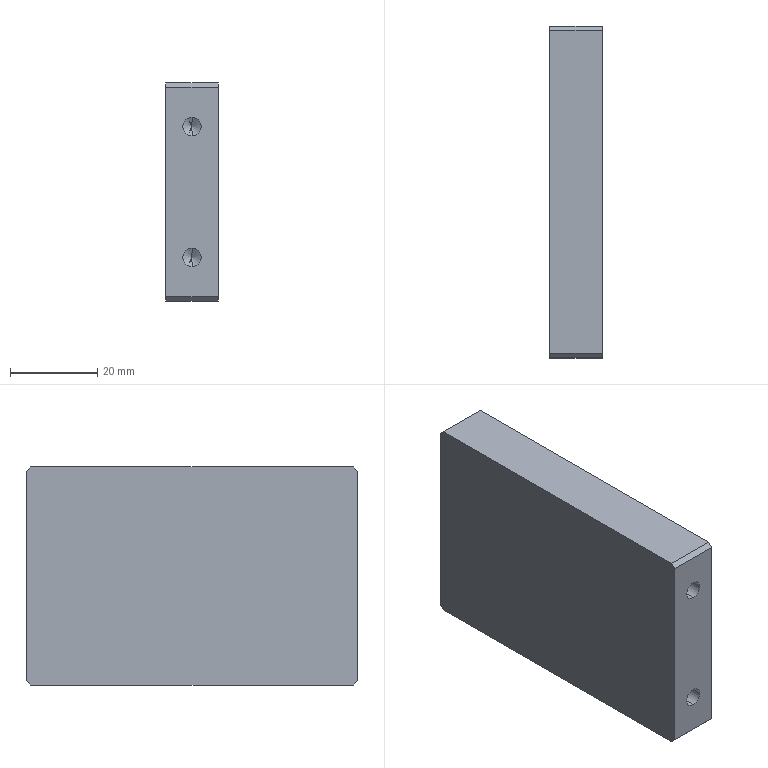Part | SolidWorks | features HoleWzd 3, Chamfer 1, ICE 1, MirrorPattern 1 | 1 solid | 26 faces | box 12 x 76 x 50 mm | volume 44588 mm3 | plane 10 | cylinder 8 | cone 8 | commonest cylinder face diameters 4.2 x8
STEP:
#1=CARTESIAN_POINT('',(-6.,20.6,-12.1));
#2=VERTEX_POINT('',#1);
#3=CARTESIAN_POINT('',(-6.,20.6,-7.9));
#4=VERTEX_POINT('',#3);
#5=CARTESIAN_POINT('',(-6.,20.6,-10.));
#6=DIRECTION('',(0.,1.,0.));
#7=DIRECTION('',(0.,0.,1.));
#8=AXIS2_PLACEMENT_3D('',#5,#6,#7);
#9=CIRCLE('',#8,2.1);
#10=EDGE_CURVE('',#2,#4,#9,.T.);
#11=ORIENTED_EDGE('',*,*,#10,.F.);
#12=CARTESIAN_POINT('',(-6.,38.,-12.1));
#13=VERTEX_POINT('',#12);
#14=CARTESIAN_POINT('',(-6.,38.,-12.1));
#15=DIRECTION('',(0.,1.,0.));
#16=VECTOR('',#15,1000.);
#17=LINE('',#14,#16);
#18=EDGE_CURVE('',#2,#13,#17,.T.);
#19=ORIENTED_EDGE('',*,*,#18,.T.);
#20=CARTESIAN_POINT('',(-6.,38.,-7.9));
#21=VERTEX_POINT('',#20);
#22=CARTESIAN_POINT('',(-6.,38.,-10.));
#23=DIRECTION('',(0.,1.,0.));
#24=DIRECTION('',(0.,0.,1.));
#25=AXIS2_PLACEMENT_3D('',#22,#23,#24);
#26=CIRCLE('',#25,2.1);
#27=EDGE_CURVE('',#13,#21,#26,.T.);
#28=ORIENTED_EDGE('',*,*,#27,.T.);
#29=CARTESIAN_POINT('',(-6.,38.,-7.9));
#30=DIRECTION('',(0.,1.,0.));
#31=VECTOR('',#30,1000.);
#32=LINE('',#29,#31);
#33=EDGE_CURVE('',#4,#21,#32,.T.);
#34=ORIENTED_EDGE('',*,*,#33,.F.);
#35=EDGE_LOOP('',(#11,#19,#28,#34));
#36=FACE_OUTER_BOUND('',#35,.T.);
#37=CARTESIAN_POINT('',(-6.,38.,-10.));
#38=DIRECTION('',(0.,1.,0.));
#39=DIRECTION('',(0.,0.,1.));
#40=AXIS2_PLACEMENT_3D('',#37,#38,#39);
#41=CYLINDRICAL_SURFACE('',#40,2.1);
#42=ADVANCED_FACE('',(#36),#41,.F.);
#43=CARTESIAN_POINT('',(-6.,19.338,-10.));
#44=VERTEX_POINT('',#43);
#45=CARTESIAN_POINT('',(-6.,20.6,-7.9));
#46=DIRECTION('',(0.,0.515,0.8572));
#47=VECTOR('',#46,1000.);
#48=LINE('',#45,#47);
#49=EDGE_CURVE('',#44,#4,#48,.T.);
#50=ORIENTED_EDGE('',*,*,#49,.F.);
#51=CARTESIAN_POINT('',(-6.,20.6,-12.1));
#52=DIRECTION('',(0.,0.515,-0.8572));
#53=VECTOR('',#52,1000.);
#54=LINE('',#51,#53);
#55=EDGE_CURVE('',#44,#2,#54,.T.);
#56=ORIENTED_EDGE('',*,*,#55,.T.);
#57=ORIENTED_EDGE('',*,*,#10,.T.);
#58=EDGE_LOOP('',(#50,#56,#57));
#59=FACE_OUTER_BOUND('',#58,.T.);
#60=CARTESIAN_POINT('',(-6.,20.6,-10.));
#61=DIRECTION('',(0.,1.,0.));
#62=DIRECTION('',(0.,0.,1.));
#63=AXIS2_PLACEMENT_3D('',#60,#61,#62);
#64=CONICAL_SURFACE('',#63,2.1,1.03);
#65=ADVANCED_FACE('',(#59),#64,.F.);
#66=CARTESIAN_POINT('',(-6.,20.6,-42.1));
#67=VERTEX_POINT('',#66);
#68=CARTESIAN_POINT('',(-6.,20.6,-37.9));
#69=VERTEX_POINT('',#68);
#70=CARTESIAN_POINT('',(-6.,20.6,-40.));
#71=DIRECTION('',(0.,1.,0.));
#72=DIRECTION('',(0.,0.,1.));
#73=AXIS2_PLACEMENT_3D('',#70,#71,#72);
#74=CIRCLE('',#73,2.1);
#75=EDGE_CURVE('',#67,#69,#74,.T.);
#76=ORIENTED_EDGE('',*,*,#75,.F.);
#77=CARTESIAN_POINT('',(-6.,38.,-42.1));
#78=VERTEX_POINT('',#77);
#79=CARTESIAN_POINT('',(-6.,38.,-42.1));
#80=DIRECTION('',(0.,1.,0.));
#81=VECTOR('',#80,1000.);
#82=LINE('',#79,#81);
#83=EDGE_CURVE('',#67,#78,#82,.T.);
#84=ORIENTED_EDGE('',*,*,#83,.T.);
#85=CARTESIAN_POINT('',(-6.,38.,-37.9));
#86=VERTEX_POINT('',#85);
#87=CARTESIAN_POINT('',(-6.,38.,-40.));
#88=DIRECTION('',(0.,1.,0.));
#89=DIRECTION('',(0.,0.,1.));
#90=AXIS2_PLACEMENT_3D('',#87,#88,#89);
#91=CIRCLE('',#90,2.1);
#92=EDGE_CURVE('',#78,#86,#91,.T.);
#93=ORIENTED_EDGE('',*,*,#92,.T.);
#94=CARTESIAN_POINT('',(-6.,38.,-37.9));
#95=DIRECTION('',(0.,1.,0.));
#96=VECTOR('',#95,1000.);
#97=LINE('',#94,#96);
#98=EDGE_CURVE('',#69,#86,#97,.T.);
#99=ORIENTED_EDGE('',*,*,#98,.F.);
#100=EDGE_LOOP('',(#76,#84,#93,#99));
#101=FACE_OUTER_BOUND('',#100,.T.);
#102=CARTESIAN_POINT('',(-6.,38.,-40.));
#103=DIRECTION('',(0.,1.,0.));
#104=DIRECTION('',(0.,0.,1.));
#105=AXIS2_PLACEMENT_3D('',#102,#103,#104);
#106=CYLINDRICAL_SURFACE('',#105,2.1);
#107=ADVANCED_FACE('',(#101),#106,.F.);
#108=CARTESIAN_POINT('',(-6.,19.338,-40.));
#109=VERTEX_POINT('',#108);
#110=CARTESIAN_POINT('',(-6.,20.6,-37.9));
#111=DIRECTION('',(0.,0.515,0.8572));
#112=VECTOR('',#111,1000.);
#113=LINE('',#110,#112);
#114=EDGE_CURVE('',#109,#69,#113,.T.);
#115=ORIENTED_EDGE('',*,*,#114,.F.);
#116=CARTESIAN_POINT('',(-6.,20.6,-42.1));
#117=DIRECTION('',(0.,0.515,-0.8572));
#118=VECTOR('',#117,1000.);
#119=LINE('',#116,#118);
#120=EDGE_CURVE('',#109,#67,#119,.T.);
#121=ORIENTED_EDGE('',*,*,#120,.T.);
#122=ORIENTED_EDGE('',*,*,#75,.T.);
#123=EDGE_LOOP('',(#115,#121,#122));
#124=FACE_OUTER_BOUND('',#123,.T.);
#125=CARTESIAN_POINT('',(-6.,20.6,-40.));
#126=DIRECTION('',(0.,1.,0.));
#127=DIRECTION('',(0.,0.,1.));
#128=AXIS2_PLACEMENT_3D('',#125,#126,#127);
#129=CONICAL_SURFACE('',#128,2.1,1.03);
#130=ADVANCED_FACE('',(#124),#129,.F.);
#131=CARTESIAN_POINT('',(-6.,-20.6,-7.9));
#132=VERTEX_POINT('',#131);
#133=CARTESIAN_POINT('',(-6.,-20.6,-12.1));
#134=VERTEX_POINT('',#133);
#135=CARTESIAN_POINT('',(-6.,-20.6,-10.));
#136=DIRECTION('',(0.,-1.,0.));
#137=DIRECTION('',(0.,0.,-1.));
#138=AXIS2_PLACEMENT_3D('',#135,#136,#137);
#139=CIRCLE('',#138,2.1);
#140=EDGE_CURVE('',#132,#134,#139,.T.);
#141=ORIENTED_EDGE('',*,*,#140,.F.);
#142=CARTESIAN_POINT('',(-6.,-38.,-7.9));
#143=VERTEX_POINT('',#142);
#144=CARTESIAN_POINT('',(-6.,-38.,-7.9));
#145=DIRECTION('',(0.,-1.,0.));
#146=VECTOR('',#145,1000.);
#147=LINE('',#144,#146);
#148=EDGE_CURVE('',#132,#143,#147,.T.);
#149=ORIENTED_EDGE('',*,*,#148,.T.);
#150=CARTESIAN_POINT('',(-6.,-38.,-12.1));
#151=VERTEX_POINT('',#150);
#152=CARTESIAN_POINT('',(-6.,-38.,-10.));
#153=DIRECTION('',(0.,-1.,0.));
#154=DIRECTION('',(0.,0.,-1.));
#155=AXIS2_PLACEMENT_3D('',#152,#153,#154);
#156=CIRCLE('',#155,2.1);
#157=EDGE_CURVE('',#143,#151,#156,.T.);
#158=ORIENTED_EDGE('',*,*,#157,.T.);
#159=CARTESIAN_POINT('',(-6.,-38.,-12.1));
#160=DIRECTION('',(0.,-1.,0.));
#161=VECTOR('',#160,1000.);
#162=LINE('',#159,#161);
#163=EDGE_CURVE('',#134,#151,#162,.T.);
#164=ORIENTED_EDGE('',*,*,#163,.F.);
#165=EDGE_LOOP('',(#141,#149,#158,#164));
#166=FACE_OUTER_BOUND('',#165,.T.);
#167=CARTESIAN_POINT('',(-6.,-38.,-10.));
#168=DIRECTION('',(0.,-1.,0.));
#169=DIRECTION('',(0.,0.,-1.));
#170=AXIS2_PLACEMENT_3D('',#167,#168,#169);
#171=CYLINDRICAL_SURFACE('',#170,2.1);
#172=ADVANCED_FACE('',(#166),#171,.F.);
#173=CARTESIAN_POINT('',(-6.,-19.338,-10.));
#174=VERTEX_POINT('',#173);
#175=CARTESIAN_POINT('',(-6.,-20.6,-12.1));
#176=DIRECTION('',(0.,-0.515,-0.8572));
#177=VECTOR('',#176,1000.);
#178=LINE('',#175,#177);
#179=EDGE_CURVE('',#174,#134,#178,.T.);
#180=ORIENTED_EDGE('',*,*,#179,.F.);
#181=CARTESIAN_POINT('',(-6.,-20.6,-7.9));
#182=DIRECTION('',(0.,-0.515,0.8572));
#183=VECTOR('',#182,1000.);
#184=LINE('',#181,#183);
#185=EDGE_CURVE('',#174,#132,#184,.T.);
#186=ORIENTED_EDGE('',*,*,#185,.T.);
#187=ORIENTED_EDGE('',*,*,#140,.T.);
#188=EDGE_LOOP('',(#180,#186,#187));
#189=FACE_OUTER_BOUND('',#188,.T.);
#190=CARTESIAN_POINT('',(-6.,-20.6,-10.));
#191=DIRECTION('',(0.,-1.,0.));
#192=DIRECTION('',(0.,0.,-1.));
#193=AXIS2_PLACEMENT_3D('',#190,#191,#192);
#194=CONICAL_SURFACE('',#193,2.1,1.03);
#195=ADVANCED_FACE('',(#189),#194,.F.);
#196=CARTESIAN_POINT('',(-6.,-20.6,-37.9));
#197=VERTEX_POINT('',#196);
#198=CARTESIAN_POINT('',(-6.,-20.6,-42.1));
#199=VERTEX_POINT('',#198);
#200=CARTESIAN_POINT('',(-6.,-20.6,-40.));
#201=DIRECTION('',(0.,-1.,0.));
#202=DIRECTION('',(0.,0.,-1.));
#203=AXIS2_PLACEMENT_3D('',#200,#201,#202);
#204=CIRCLE('',#203,2.1);
#205=EDGE_CURVE('',#197,#199,#204,.T.);
#206=ORIENTED_EDGE('',*,*,#205,.F.);
#207=CARTESIAN_POINT('',(-6.,-38.,-37.9));
#208=VERTEX_POINT('',#207);
#209=CARTESIAN_POINT('',(-6.,-38.,-37.9));
#210=DIRECTION('',(0.,-1.,0.));
#211=VECTOR('',#210,1000.);
#212=LINE('',#209,#211);
#213=EDGE_CURVE('',#197,#208,#212,.T.);
#214=ORIENTED_EDGE('',*,*,#213,.T.);
#215=CARTESIAN_POINT('',(-6.,-38.,-42.1));
#216=VERTEX_POINT('',#215);
#217=CARTESIAN_POINT('',(-6.,-38.,-40.));
#218=DIRECTION('',(0.,-1.,0.));
#219=DIRECTION('',(0.,0.,-1.));
#220=AXIS2_PLACEMENT_3D('',#217,#218,#219);
#221=CIRCLE('',#220,2.1);
#222=EDGE_CURVE('',#208,#216,#221,.T.);
#223=ORIENTED_EDGE('',*,*,#222,.T.);
#224=CARTESIAN_POINT('',(-6.,-38.,-42.1));
#225=DIRECTION('',(0.,-1.,0.));
#226=VECTOR('',#225,1000.);
#227=LINE('',#224,#226);
#228=EDGE_CURVE('',#199,#216,#227,.T.);
#229=ORIENTED_EDGE('',*,*,#228,.F.);
#230=EDGE_LOOP('',(#206,#214,#223,#229));
#231=FACE_OUTER_BOUND('',#230,.T.);
#232=CARTESIAN_POINT('',(-6.,-38.,-40.));
#233=DIRECTION('',(0.,-1.,0.));
#234=DIRECTION('',(0.,0.,-1.));
#235=AXIS2_PLACEMENT_3D('',#232,#233,#234);
#236=CYLINDRICAL_SURFACE('',#235,2.1);
#237=ADVANCED_FACE('',(#231),#236,.F.);
#238=CARTESIAN_POINT('',(-6.,-19.338,-40.));
#239=VERTEX_POINT('',#238);
#240=CARTESIAN_POINT('',(-6.,-20.6,-42.1));
#241=DIRECTION('',(0.,-0.515,-0.8572));
#242=VECTOR('',#241,1000.);
#243=LINE('',#240,#242);
#244=EDGE_CURVE('',#239,#199,#243,.T.);
#245=ORIENTED_EDGE('',*,*,#244,.F.);
#246=CARTESIAN_POINT('',(-6.,-20.6,-37.9));
#247=DIRECTION('',(0.,-0.515,0.8572));
#248=VECTOR('',#247,1000.);
#249=LINE('',#246,#248);
#250=EDGE_CURVE('',#239,#197,#249,.T.);
#251=ORIENTED_EDGE('',*,*,#250,.T.);
#252=ORIENTED_EDGE('',*,*,#205,.T.);
#253=EDGE_LOOP('',(#245,#251,#252));
#254=FACE_OUTER_BOUND('',#253,.T.);
#255=CARTESIAN_POINT('',(-6.,-20.6,-40.));
#256=DIRECTION('',(0.,-1.,0.));
#257=DIRECTION('',(0.,0.,-1.));
#258=AXIS2_PLACEMENT_3D('',#255,#256,#257);
#259=CONICAL_SURFACE('',#258,2.1,1.03);
#260=ADVANCED_FACE('',(#254),#259,.F.);
#261=CARTESIAN_POINT('',(0.,37.,0.));
#262=VERTEX_POINT('',#261);
#263=CARTESIAN_POINT('',(0.,-37.,0.));
#264=VERTEX_POINT('',#263);
#265=CARTESIAN_POINT('',(0.,38.,0.));
#266=DIRECTION('',(0.,-1.,0.));
#267=VECTOR('',#266,1000.);
#268=LINE('',#265,#267);
#269=EDGE_CURVE('',#262,#264,#268,.T.);
#270=ORIENTED_EDGE('',*,*,#269,.F.);
#271=CARTESIAN_POINT('',(-12.,37.,0.));
#272=VERTEX_POINT('',#271);
#273=CARTESIAN_POINT('',(-12.,37.,0.));
#274=DIRECTION('',(-1.,0.,0.));
#275=VECTOR('',#274,1000.);
#276=LINE('',#273,#275);
#277=EDGE_CURVE('',#262,#272,#276,.T.);
#278=ORIENTED_EDGE('',*,*,#277,.T.);
#279=CARTESIAN_POINT('',(-12.,-37.,0.));
#280=VERTEX_POINT('',#279);
#281=CARTESIAN_POINT('',(-12.,38.,0.));
#282=DIRECTION('',(0.,-1.,0.));
#283=VECTOR('',#282,1000.);
#284=LINE('',#281,#283);
#285=EDGE_CURVE('',#272,#280,#284,.T.);
#286=ORIENTED_EDGE('',*,*,#285,.T.);
#287=CARTESIAN_POINT('',(-12.,-37.,0.));
#288=DIRECTION('',(1.,0.,0.));
#289=VECTOR('',#288,1000.);
#290=LINE('',#287,#289);
#291=EDGE_CURVE('',#280,#264,#290,.T.);
#292=ORIENTED_EDGE('',*,*,#291,.T.);
#293=EDGE_LOOP('',(#270,#278,#286,#292));
#294=FACE_OUTER_BOUND('',#293,.T.);
#295=CARTESIAN_POINT('',(-12.,38.,0.));
#296=DIRECTION('',(0.,0.,1.));
#297=DIRECTION('',(1.,0.,0.));
#298=AXIS2_PLACEMENT_3D('',#295,#296,#297);
#299=PLANE('',#298);
#300=ADVANCED_FACE('',(#294),#299,.T.);
#301=CARTESIAN_POINT('',(-6.,38.,-10.));
#302=DIRECTION('',(0.,1.,0.));
#303=DIRECTION('',(0.,0.,1.));
#304=AXIS2_PLACEMENT_3D('',#301,#302,#303);
#305=CIRCLE('',#304,2.1);
#306=EDGE_CURVE('',#21,#13,#305,.T.);
#307=ORIENTED_EDGE('',*,*,#306,.F.);
#308=ORIENTED_EDGE('',*,*,#27,.F.);
#309=EDGE_LOOP('',(#307,#308));
#310=FACE_BOUND('',#309,.T.);
#311=CARTESIAN_POINT('',(-6.,38.,-40.));
#312=DIRECTION('',(0.,1.,0.));
#313=DIRECTION('',(0.,0.,1.));
#314=AXIS2_PLACEMENT_3D('',#311,#312,#313);
#315=CIRCLE('',#314,2.1);
#316=EDGE_CURVE('',#86,#78,#315,.T.);
#317=ORIENTED_EDGE('',*,*,#316,.F.);
#318=ORIENTED_EDGE('',*,*,#92,.F.);
#319=EDGE_LOOP('',(#317,#318));
#320=FACE_BOUND('',#319,.T.);
#321=CARTESIAN_POINT('',(-12.,38.,-49.));
#322=VERTEX_POINT('',#321);
#323=CARTESIAN_POINT('',(-12.,38.,-1.));
#324=VERTEX_POINT('',#323);
#325=CARTESIAN_POINT('',(-12.,38.,0.));
#326=DIRECTION('',(0.,0.,1.));
#327=VECTOR('',#326,1000.);
#328=LINE('',#325,#327);
#329=EDGE_CURVE('',#322,#324,#328,.T.);
#330=ORIENTED_EDGE('',*,*,#329,.T.);
#331=CARTESIAN_POINT('',(0.,38.,-1.));
#332=VERTEX_POINT('',#331);
#333=CARTESIAN_POINT('',(-12.,38.,-1.));
#334=DIRECTION('',(1.,0.,0.));
#335=VECTOR('',#334,1000.);
#336=LINE('',#333,#335);
#337=EDGE_CURVE('',#324,#332,#336,.T.);
#338=ORIENTED_EDGE('',*,*,#337,.T.);
#339=CARTESIAN_POINT('',(0.,38.,-49.));
#340=VERTEX_POINT('',#339);
#341=CARTESIAN_POINT('',(0.,38.,0.));
#342=DIRECTION('',(0.,0.,1.));
#343=VECTOR('',#342,1000.);
#344=LINE('',#341,#343);
#345=EDGE_CURVE('',#340,#332,#344,.T.);
#346=ORIENTED_EDGE('',*,*,#345,.F.);
#347=CARTESIAN_POINT('',(-12.,38.,-49.));
#348=DIRECTION('',(-1.,0.,0.));
#349=VECTOR('',#348,1000.);
#350=LINE('',#347,#349);
#351=EDGE_CURVE('',#340,#322,#350,.T.);
#352=ORIENTED_EDGE('',*,*,#351,.T.);
#353=EDGE_LOOP('',(#330,#338,#346,#352));
#354=FACE_OUTER_BOUND('',#353,.T.);
#355=CARTESIAN_POINT('',(-12.,38.,0.));
#356=DIRECTION('',(0.,1.,0.));
#357=DIRECTION('',(0.,0.,1.));
#358=AXIS2_PLACEMENT_3D('',#355,#356,#357);
#359=PLANE('',#358);
#360=ADVANCED_FACE('',(#310,#320,#354),#359,.T.);
#361=CARTESIAN_POINT('',(-12.,-37.,-50.));
#362=VERTEX_POINT('',#361);
#363=CARTESIAN_POINT('',(-12.,37.,-50.));
#364=VERTEX_POINT('',#363);
#365=CARTESIAN_POINT('',(-12.,38.,-50.));
#366=DIRECTION('',(0.,1.,0.));
#367=VECTOR('',#366,1000.);
#368=LINE('',#365,#367);
#369=EDGE_CURVE('',#362,#364,#368,.T.);
#370=ORIENTED_EDGE('',*,*,#369,.T.);
#371=CARTESIAN_POINT('',(0.,37.,-50.));
#372=VERTEX_POINT('',#371);
#373=CARTESIAN_POINT('',(-12.,37.,-50.));
#374=DIRECTION('',(1.,0.,0.));
#375=VECTOR('',#374,1000.);
#376=LINE('',#373,#375);
#377=EDGE_CURVE('',#364,#372,#376,.T.);
#378=ORIENTED_EDGE('',*,*,#377,.T.);
#379=CARTESIAN_POINT('',(0.,-37.,-50.));
#380=VERTEX_POINT('',#379);
#381=CARTESIAN_POINT('',(0.,38.,-50.));
#382=DIRECTION('',(0.,1.,0.));
#383=VECTOR('',#382,1000.);
#384=LINE('',#381,#383);
#385=EDGE_CURVE('',#380,#372,#384,.T.);
#386=ORIENTED_EDGE('',*,*,#385,.F.);
#387=CARTESIAN_POINT('',(-12.,-37.,-50.));
#388=DIRECTION('',(-1.,0.,0.));
#389=VECTOR('',#388,1000.);
#390=LINE('',#387,#389);
#391=EDGE_CURVE('',#380,#362,#390,.T.);
#392=ORIENTED_EDGE('',*,*,#391,.T.);
#393=EDGE_LOOP('',(#370,#378,#386,#392));
#394=FACE_OUTER_BOUND('',#393,.T.);
#395=CARTESIAN_POINT('',(-12.,38.,-50.));
#396=DIRECTION('',(0.,0.,-1.));
#397=DIRECTION('',(-1.,0.,0.));
#398=AXIS2_PLACEMENT_3D('',#395,#396,#397);
#399=PLANE('',#398);
#400=ADVANCED_FACE('',(#394),#399,.T.);
#401=CARTESIAN_POINT('',(-6.,-38.,-10.));
#402=DIRECTION('',(0.,-1.,0.));
#403=DIRECTION('',(0.,0.,-1.));
#404=AXIS2_PLACEMENT_3D('',#401,#402,#403);
#405=CIRCLE('',#404,2.1);
#406=EDGE_CURVE('',#151,#143,#405,.T.);
#407=ORIENTED_EDGE('',*,*,#406,.F.);
#408=ORIENTED_EDGE('',*,*,#157,.F.);
#409=EDGE_LOOP('',(#407,#408));
#410=FACE_BOUND('',#409,.T.);
#411=CARTESIAN_POINT('',(-6.,-38.,-40.));
#412=DIRECTION('',(0.,-1.,0.));
#413=DIRECTION('',(0.,0.,-1.));
#414=AXIS2_PLACEMENT_3D('',#411,#412,#413);
#415=CIRCLE('',#414,2.1);
#416=EDGE_CURVE('',#216,#208,#415,.T.);
#417=ORIENTED_EDGE('',*,*,#416,.F.);
#418=ORIENTED_EDGE('',*,*,#222,.F.);
#419=EDGE_LOOP('',(#417,#418));
#420=FACE_BOUND('',#419,.T.);
#421=CARTESIAN_POINT('',(-12.,-38.,-1.));
#422=VERTEX_POINT('',#421);
#423=CARTESIAN_POINT('',(-12.,-38.,-49.));
#424=VERTEX_POINT('',#423);
#425=CARTESIAN_POINT('',(-12.,-38.,0.));
#426=DIRECTION('',(0.,0.,-1.));
#427=VECTOR('',#426,1000.);
#428=LINE('',#425,#427);
#429=EDGE_CURVE('',#422,#424,#428,.T.);
#430=ORIENTED_EDGE('',*,*,#429,.T.);
#431=CARTESIAN_POINT('',(0.,-38.,-49.));
#432=VERTEX_POINT('',#431);
#433=CARTESIAN_POINT('',(-12.,-38.,-49.));
#434=DIRECTION('',(1.,0.,0.));
#435=VECTOR('',#434,1000.);
#436=LINE('',#433,#435);
#437=EDGE_CURVE('',#424,#432,#436,.T.);
#438=ORIENTED_EDGE('',*,*,#437,.T.);
#439=CARTESIAN_POINT('',(0.,-38.,-1.));
#440=VERTEX_POINT('',#439);
#441=CARTESIAN_POINT('',(0.,-38.,0.));
#442=DIRECTION('',(0.,0.,-1.));
#443=VECTOR('',#442,1000.);
#444=LINE('',#441,#443);
#445=EDGE_CURVE('',#440,#432,#444,.T.);
#446=ORIENTED_EDGE('',*,*,#445,.F.);
#447=CARTESIAN_POINT('',(-12.,-38.,-1.));
#448=DIRECTION('',(-1.,0.,0.));
#449=VECTOR('',#448,1000.);
#450=LINE('',#447,#449);
#451=EDGE_CURVE('',#440,#422,#450,.T.);
#452=ORIENTED_EDGE('',*,*,#451,.T.);
#453=EDGE_LOOP('',(#430,#438,#446,#452));
#454=FACE_OUTER_BOUND('',#453,.T.);
#455=CARTESIAN_POINT('',(-12.,-38.,0.));
#456=DIRECTION('',(0.,-1.,0.));
#457=DIRECTION('',(0.,0.,-1.));
#458=AXIS2_PLACEMENT_3D('',#455,#456,#457);
#459=PLANE('',#458);
#460=ADVANCED_FACE('',(#410,#420,#454),#459,.T.);
#461=ORIENTED_EDGE('',*,*,#285,.F.);
#462=CARTESIAN_POINT('',(-12.,38.,-1.));
#463=DIRECTION('',(0.,0.7071,-0.7071));
#464=VECTOR('',#463,1000.);
#465=LINE('',#462,#464);
#466=EDGE_CURVE('',#272,#324,#465,.T.);
#467=ORIENTED_EDGE('',*,*,#466,.T.);
#468=ORIENTED_EDGE('',*,*,#329,.F.);
#469=CARTESIAN_POINT('',(-12.,37.,-50.));
#470=DIRECTION('',(0.,-0.7071,-0.7071));
#471=VECTOR('',#470,1000.);
#472=LINE('',#469,#471);
#473=EDGE_CURVE('',#322,#364,#472,.T.);
#474=ORIENTED_EDGE('',*,*,#473,.T.);
#475=ORIENTED_EDGE('',*,*,#369,.F.);
#476=CARTESIAN_POINT('',(-12.,-38.,-49.));
#477=DIRECTION('',(0.,-0.7071,0.7071));
#478=VECTOR('',#477,1000.);
#479=LINE('',#476,#478);
#480=EDGE_CURVE('',#362,#424,#479,.T.);
#481=ORIENTED_EDGE('',*,*,#480,.T.);
#482=ORIENTED_EDGE('',*,*,#429,.F.);
#483=CARTESIAN_POINT('',(-12.,-37.,0.));
#484=DIRECTION('',(0.,0.7071,0.7071));
#485=VECTOR('',#484,1000.);
#486=LINE('',#483,#485);
#487=EDGE_CURVE('',#422,#280,#486,.T.);
#488=ORIENTED_EDGE('',*,*,#487,.T.);
#489=EDGE_LOOP('',(#461,#467,#468,#474,#475,#481,#482,#488));
#490=FACE_OUTER_BOUND('',#489,.T.);
#491=CARTESIAN_POINT('',(-12.,0.,0.));
#492=DIRECTION('',(1.,0.,0.));
#493=DIRECTION('',(0.,0.,-1.));
#494=AXIS2_PLACEMENT_3D('',#491,#492,#493);
#495=PLANE('',#494);
#496=ADVANCED_FACE('',(#490),#495,.F.);
#497=ORIENTED_EDGE('',*,*,#345,.T.);
#498=CARTESIAN_POINT('',(0.,18.5,18.5));
#499=DIRECTION('',(0.,-0.7071,0.7071));
#500=VECTOR('',#499,1000.);
#501=LINE('',#498,#500);
#502=EDGE_CURVE('',#332,#262,#501,.T.);
#503=ORIENTED_EDGE('',*,*,#502,.T.);
#504=ORIENTED_EDGE('',*,*,#269,.T.);
#505=CARTESIAN_POINT('',(0.,-18.5,18.5));
#506=DIRECTION('',(0.,-0.7071,-0.7071));
#507=VECTOR('',#506,1000.);
#508=LINE('',#505,#507);
#509=EDGE_CURVE('',#264,#440,#508,.T.);
#510=ORIENTED_EDGE('',*,*,#509,.T.);
#511=ORIENTED_EDGE('',*,*,#445,.T.);
#512=CARTESIAN_POINT('',(0.,-43.5,-43.5));
#513=DIRECTION('',(0.,0.7071,-0.7071));
#514=VECTOR('',#513,1000.);
#515=LINE('',#512,#514);
#516=EDGE_CURVE('',#432,#380,#515,.T.);
#517=ORIENTED_EDGE('',*,*,#516,.T.);
#518=ORIENTED_EDGE('',*,*,#385,.T.);
#519=CARTESIAN_POINT('',(0.,43.5,-43.5));
#520=DIRECTION('',(0.,0.7071,0.7071));
#521=VECTOR('',#520,1000.);
#522=LINE('',#519,#521);
#523=EDGE_CURVE('',#372,#340,#522,.T.);
#524=ORIENTED_EDGE('',*,*,#523,.T.);
#525=EDGE_LOOP('',(#497,#503,#504,#510,#511,#517,#518,#524));
#526=FACE_OUTER_BOUND('',#525,.T.);
#527=CARTESIAN_POINT('',(0.,0.,0.));
#528=DIRECTION('',(1.,0.,0.));
#529=DIRECTION('',(0.,0.,-1.));
#530=AXIS2_PLACEMENT_3D('',#527,#528,#529);
#531=PLANE('',#530);
#532=ADVANCED_FACE('',(#526),#531,.T.);
#533=ORIENTED_EDGE('',*,*,#250,.F.);
#534=ORIENTED_EDGE('',*,*,#244,.T.);
#535=CARTESIAN_POINT('',(-6.,-20.6,-40.));
#536=DIRECTION('',(0.,-1.,0.));
#537=DIRECTION('',(0.,0.,-1.));
#538=AXIS2_PLACEMENT_3D('',#535,#536,#537);
#539=CIRCLE('',#538,2.1);
#540=EDGE_CURVE('',#199,#197,#539,.T.);
#541=ORIENTED_EDGE('',*,*,#540,.T.);
#542=EDGE_LOOP('',(#533,#534,#541));
#543=FACE_OUTER_BOUND('',#542,.T.);
#544=CARTESIAN_POINT('',(-6.,-20.6,-40.));
#545=DIRECTION('',(0.,-1.,0.));
#546=DIRECTION('',(0.,0.,-1.));
#547=AXIS2_PLACEMENT_3D('',#544,#545,#546);
#548=CONICAL_SURFACE('',#547,2.1,1.03);
#549=ADVANCED_FACE('',(#543),#548,.F.);
#550=ORIENTED_EDGE('',*,*,#213,.F.);
#551=ORIENTED_EDGE('',*,*,#540,.F.);
#552=ORIENTED_EDGE('',*,*,#228,.T.);
#553=ORIENTED_EDGE('',*,*,#416,.T.);
#554=EDGE_LOOP('',(#550,#551,#552,#553));
#555=FACE_OUTER_BOUND('',#554,.T.);
#556=CARTESIAN_POINT('',(-6.,-38.,-40.));
#557=DIRECTION('',(0.,-1.,0.));
#558=DIRECTION('',(0.,0.,-1.));
#559=AXIS2_PLACEMENT_3D('',#556,#557,#558);
#560=CYLINDRICAL_SURFACE('',#559,2.1);
#561=ADVANCED_FACE('',(#555),#560,.F.);
#562=ORIENTED_EDGE('',*,*,#185,.F.);
#563=ORIENTED_EDGE('',*,*,#179,.T.);
#564=CARTESIAN_POINT('',(-6.,-20.6,-10.));
#565=DIRECTION('',(0.,-1.,0.));
#566=DIRECTION('',(0.,0.,-1.));
#567=AXIS2_PLACEMENT_3D('',#564,#565,#566);
#568=CIRCLE('',#567,2.1);
#569=EDGE_CURVE('',#134,#132,#568,.T.);
#570=ORIENTED_EDGE('',*,*,#569,.T.);
#571=EDGE_LOOP('',(#562,#563,#570));
#572=FACE_OUTER_BOUND('',#571,.T.);
#573=CARTESIAN_POINT('',(-6.,-20.6,-10.));
#574=DIRECTION('',(0.,-1.,0.));
#575=DIRECTION('',(0.,0.,-1.));
#576=AXIS2_PLACEMENT_3D('',#573,#574,#575);
#577=CONICAL_SURFACE('',#576,2.1,1.03);
#578=ADVANCED_FACE('',(#572),#577,.F.);
#579=ORIENTED_EDGE('',*,*,#148,.F.);
#580=ORIENTED_EDGE('',*,*,#569,.F.);
#581=ORIENTED_EDGE('',*,*,#163,.T.);
#582=ORIENTED_EDGE('',*,*,#406,.T.);
#583=EDGE_LOOP('',(#579,#580,#581,#582));
#584=FACE_OUTER_BOUND('',#583,.T.);
#585=CARTESIAN_POINT('',(-6.,-38.,-10.));
#586=DIRECTION('',(0.,-1.,0.));
#587=DIRECTION('',(0.,0.,-1.));
#588=AXIS2_PLACEMENT_3D('',#585,#586,#587);
#589=CYLINDRICAL_SURFACE('',#588,2.1);
#590=ADVANCED_FACE('',(#584),#589,.F.);
#591=ORIENTED_EDGE('',*,*,#120,.F.);
#592=ORIENTED_EDGE('',*,*,#114,.T.);
#593=CARTESIAN_POINT('',(-6.,20.6,-40.));
#594=DIRECTION('',(0.,1.,0.));
#595=DIRECTION('',(0.,0.,1.));
#596=AXIS2_PLACEMENT_3D('',#593,#594,#595);
#597=CIRCLE('',#596,2.1);
#598=EDGE_CURVE('',#69,#67,#597,.T.);
#599=ORIENTED_EDGE('',*,*,#598,.T.);
#600=EDGE_LOOP('',(#591,#592,#599));
#601=FACE_OUTER_BOUND('',#600,.T.);
#602=CARTESIAN_POINT('',(-6.,20.6,-40.));
#603=DIRECTION('',(0.,1.,0.));
#604=DIRECTION('',(0.,0.,1.));
#605=AXIS2_PLACEMENT_3D('',#602,#603,#604);
#606=CONICAL_SURFACE('',#605,2.1,1.03);
#607=ADVANCED_FACE('',(#601),#606,.F.);
#608=ORIENTED_EDGE('',*,*,#83,.F.);
#609=ORIENTED_EDGE('',*,*,#598,.F.);
#610=ORIENTED_EDGE('',*,*,#98,.T.);
#611=ORIENTED_EDGE('',*,*,#316,.T.);
#612=EDGE_LOOP('',(#608,#609,#610,#611));
#613=FACE_OUTER_BOUND('',#612,.T.);
#614=CARTESIAN_POINT('',(-6.,38.,-40.));
#615=DIRECTION('',(0.,1.,0.));
#616=DIRECTION('',(0.,0.,1.));
#617=AXIS2_PLACEMENT_3D('',#614,#615,#616);
#618=CYLINDRICAL_SURFACE('',#617,2.1);
#619=ADVANCED_FACE('',(#613),#618,.F.);
#620=ORIENTED_EDGE('',*,*,#55,.F.);
#621=ORIENTED_EDGE('',*,*,#49,.T.);
#622=CARTESIAN_POINT('',(-6.,20.6,-10.));
#623=DIRECTION('',(0.,1.,0.));
#624=DIRECTION('',(0.,0.,1.));
#625=AXIS2_PLACEMENT_3D('',#622,#623,#624);
#626=CIRCLE('',#625,2.1);
#627=EDGE_CURVE('',#4,#2,#626,.T.);
#628=ORIENTED_EDGE('',*,*,#627,.T.);
#629=EDGE_LOOP('',(#620,#621,#628));
#630=FACE_OUTER_BOUND('',#629,.T.);
#631=CARTESIAN_POINT('',(-6.,20.6,-10.));
#632=DIRECTION('',(0.,1.,0.));
#633=DIRECTION('',(0.,0.,1.));
#634=AXIS2_PLACEMENT_3D('',#631,#632,#633);
#635=CONICAL_SURFACE('',#634,2.1,1.03);
#636=ADVANCED_FACE('',(#630),#635,.F.);
#637=ORIENTED_EDGE('',*,*,#18,.F.);
#638=ORIENTED_EDGE('',*,*,#627,.F.);
#639=ORIENTED_EDGE('',*,*,#33,.T.);
#640=ORIENTED_EDGE('',*,*,#306,.T.);
#641=EDGE_LOOP('',(#637,#638,#639,#640));
#642=FACE_OUTER_BOUND('',#641,.T.);
#643=CARTESIAN_POINT('',(-6.,38.,-10.));
#644=DIRECTION('',(0.,1.,0.));
#645=DIRECTION('',(0.,0.,1.));
#646=AXIS2_PLACEMENT_3D('',#643,#644,#645);
#647=CYLINDRICAL_SURFACE('',#646,2.1);
#648=ADVANCED_FACE('',(#642),#647,.F.);
#649=ORIENTED_EDGE('',*,*,#466,.F.);
#650=ORIENTED_EDGE('',*,*,#277,.F.);
#651=ORIENTED_EDGE('',*,*,#502,.F.);
#652=ORIENTED_EDGE('',*,*,#337,.F.);
#653=EDGE_LOOP('',(#649,#650,#651,#652));
#654=FACE_OUTER_BOUND('',#653,.T.);
#655=CARTESIAN_POINT('',(-12.,38.,-1.));
#656=DIRECTION('',(0.,-0.7071,-0.7071));
#657=DIRECTION('',(1.,0.,0.));
#658=AXIS2_PLACEMENT_3D('',#655,#656,#657);
#659=PLANE('',#658);
#660=ADVANCED_FACE('',(#654),#659,.F.);
#661=ORIENTED_EDGE('',*,*,#473,.F.);
#662=ORIENTED_EDGE('',*,*,#351,.F.);
#663=ORIENTED_EDGE('',*,*,#523,.F.);
#664=ORIENTED_EDGE('',*,*,#377,.F.);
#665=EDGE_LOOP('',(#661,#662,#663,#664));
#666=FACE_OUTER_BOUND('',#665,.T.);
#667=CARTESIAN_POINT('',(-12.,37.,-50.));
#668=DIRECTION('',(0.,-0.7071,0.7071));
#669=DIRECTION('',(1.,0.,0.));
#670=AXIS2_PLACEMENT_3D('',#667,#668,#669);
#671=PLANE('',#670);
#672=ADVANCED_FACE('',(#666),#671,.F.);
#673=ORIENTED_EDGE('',*,*,#480,.F.);
#674=ORIENTED_EDGE('',*,*,#391,.F.);
#675=ORIENTED_EDGE('',*,*,#516,.F.);
#676=ORIENTED_EDGE('',*,*,#437,.F.);
#677=EDGE_LOOP('',(#673,#674,#675,#676));
#678=FACE_OUTER_BOUND('',#677,.T.);
#679=CARTESIAN_POINT('',(-12.,-38.,-49.));
#680=DIRECTION('',(0.,0.7071,0.7071));
#681=DIRECTION('',(1.,0.,0.));
#682=AXIS2_PLACEMENT_3D('',#679,#680,#681);
#683=PLANE('',#682);
#684=ADVANCED_FACE('',(#678),#683,.F.);
#685=ORIENTED_EDGE('',*,*,#487,.F.);
#686=ORIENTED_EDGE('',*,*,#451,.F.);
#687=ORIENTED_EDGE('',*,*,#509,.F.);
#688=ORIENTED_EDGE('',*,*,#291,.F.);
#689=EDGE_LOOP('',(#685,#686,#687,#688));
#690=FACE_OUTER_BOUND('',#689,.T.);
#691=CARTESIAN_POINT('',(-12.,-37.,0.));
#692=DIRECTION('',(0.,0.7071,-0.7071));
#693=DIRECTION('',(1.,0.,0.));
#694=AXIS2_PLACEMENT_3D('',#691,#692,#693);
#695=PLANE('',#694);
#696=ADVANCED_FACE('',(#690),#695,.F.);
#697=CLOSED_SHELL('',(#42,#65,#107,#130,#172,#195,#237,#260,#300,#360,#400,#460,#496,#532,#549,#561,#578,#590,#607,#619,#636,#648,#660,#672,#684,#696));
#698=MANIFOLD_SOLID_BREP('',#697);
#699=CARTESIAN_POINT('',(0.,0.,0.));
#700=DIRECTION('',(0.,0.,1.));
#701=DIRECTION('',(1.,0.,0.));
#702=AXIS2_PLACEMENT_3D('',#699,#700,#701);
#703=(LENGTH_UNIT()NAMED_UNIT(*)SI_UNIT(.MILLI.,.METRE.));
#704=UNCERTAINTY_MEASURE_WITH_UNIT(LENGTH_MEASURE(0.00001),#703,'','');
#705=(NAMED_UNIT(*)PLANE_ANGLE_UNIT()SI_UNIT($,.RADIAN.));
#706=(NAMED_UNIT(*)SI_UNIT($,.STERADIAN.)SOLID_ANGLE_UNIT());
#707=(GEOMETRIC_REPRESENTATION_CONTEXT(3)GLOBAL_UNCERTAINTY_ASSIGNED_CONTEXT((#704))GLOBAL_UNIT_ASSIGNED_CONTEXT((#703,#705,#706))REPRESENTATION_CONTEXT('',''));
#708=ADVANCED_BREP_SHAPE_REPRESENTATION('',(#698,#702),#707);